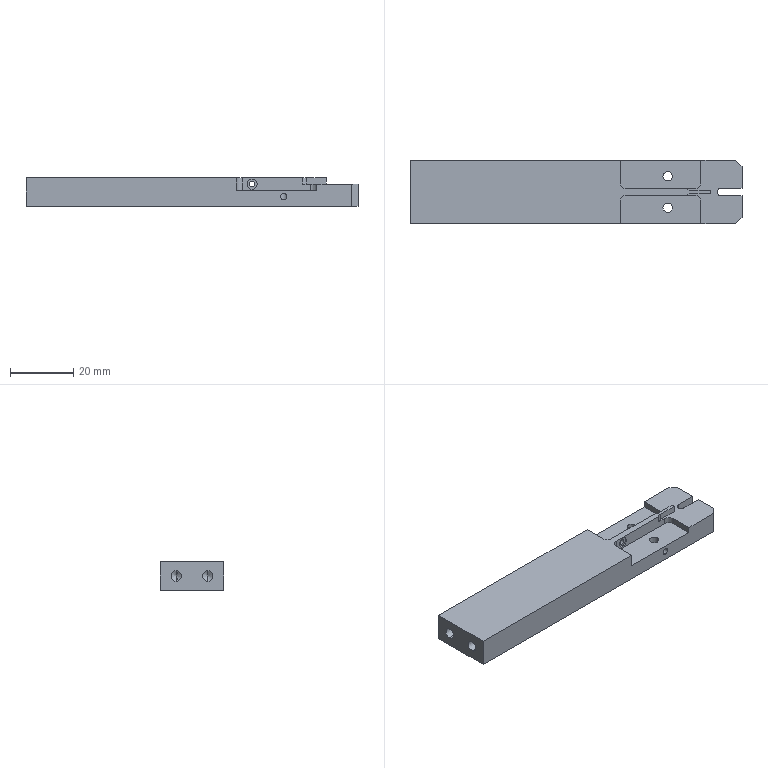Part | STEP file | BU-B04 | 1 solid | 60 faces | box 105 x 20 x 9 mm | volume 16085 mm3 | cylinder 28 | plane 28 | cone 4 | commonest cylinder face diameters 4 x6 2.05 x4 3 x4 3.2 x4 3.3 x4 1.8 x2